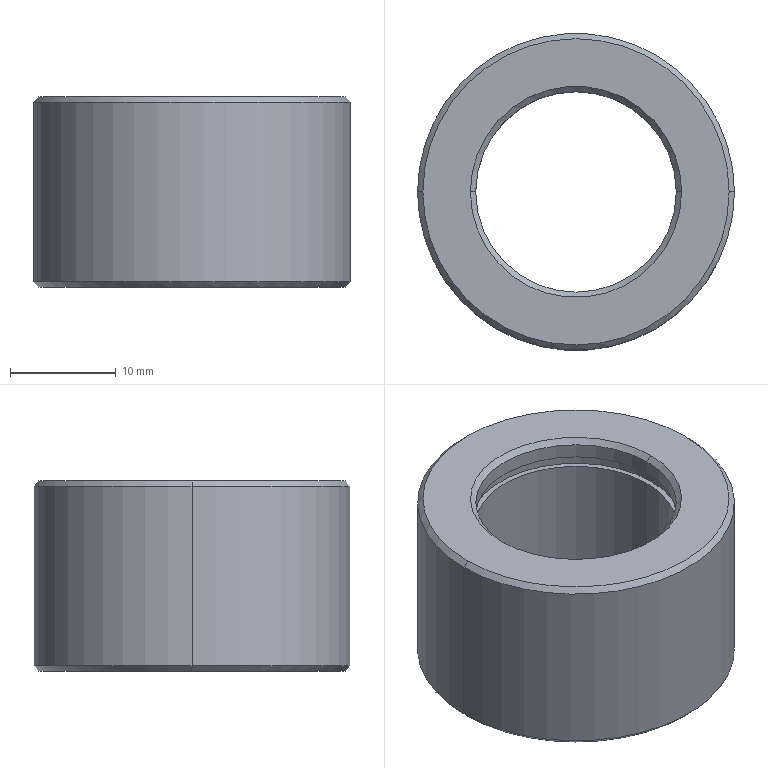Part | SolidWorks | features Chamfer 1, Extrusion 1, ICE 1, MirrorPattern 1 | 1 solid | 26 faces | box 30 x 30 x 18 mm | volume 7514 mm3 | cylinder 12 | cone 8 | plane 6 | commonest cylinder face diameters 19 x6 20 x4 30 x2
STEP:
#1=CARTESIAN_POINT('',(-9.5,0.,8.5));
#2=VERTEX_POINT('',#1);
#3=CARTESIAN_POINT('',(9.5,0.,8.5));
#4=VERTEX_POINT('',#3);
#5=CARTESIAN_POINT('',(0.,0.,8.5));
#6=DIRECTION('',(0.,0.,1.));
#7=DIRECTION('',(1.,0.,0.));
#8=AXIS2_PLACEMENT_3D('',#5,#6,#7);
#9=CIRCLE('',#8,9.5);
#10=EDGE_CURVE('',#2,#4,#9,.T.);
#11=ORIENTED_EDGE('',*,*,#10,.F.);
#12=CARTESIAN_POINT('',(-10.,0.,9.));
#13=VERTEX_POINT('',#12);
#14=CARTESIAN_POINT('',(-9.5,0.,8.5));
#15=DIRECTION('',(-0.7071,0.,0.7071));
#16=VECTOR('',#15,1000.);
#17=LINE('',#14,#16);
#18=EDGE_CURVE('',#2,#13,#17,.T.);
#19=ORIENTED_EDGE('',*,*,#18,.T.);
#20=CARTESIAN_POINT('',(10.,0.,9.));
#21=VERTEX_POINT('',#20);
#22=CARTESIAN_POINT('',(0.,0.,9.));
#23=DIRECTION('',(0.,0.,-1.));
#24=DIRECTION('',(1.,0.,0.));
#25=AXIS2_PLACEMENT_3D('',#22,#23,#24);
#26=CIRCLE('',#25,10.);
#27=EDGE_CURVE('',#21,#13,#26,.T.);
#28=ORIENTED_EDGE('',*,*,#27,.F.);
#29=CARTESIAN_POINT('',(9.5,0.,8.5));
#30=DIRECTION('',(0.7071,0.,0.7071));
#31=VECTOR('',#30,1000.);
#32=LINE('',#29,#31);
#33=EDGE_CURVE('',#4,#21,#32,.T.);
#34=ORIENTED_EDGE('',*,*,#33,.F.);
#35=EDGE_LOOP('',(#11,#19,#28,#34));
#36=FACE_OUTER_BOUND('',#35,.T.);
#37=CARTESIAN_POINT('',(0.,0.,8.5));
#38=DIRECTION('',(0.,0.,1.));
#39=DIRECTION('',(1.,0.,0.));
#40=AXIS2_PLACEMENT_3D('',#37,#38,#39);
#41=CONICAL_SURFACE('',#40,9.5,0.7854);
#42=ADVANCED_FACE('',(#36),#41,.F.);
#43=CARTESIAN_POINT('',(9.5,0.,-8.5));
#44=VERTEX_POINT('',#43);
#45=CARTESIAN_POINT('',(-9.5,0.,-8.5));
#46=VERTEX_POINT('',#45);
#47=CARTESIAN_POINT('',(0.,0.,-8.5));
#48=DIRECTION('',(0.,0.,-1.));
#49=DIRECTION('',(1.,0.,0.));
#50=AXIS2_PLACEMENT_3D('',#47,#48,#49);
#51=CIRCLE('',#50,9.5);
#52=EDGE_CURVE('',#44,#46,#51,.T.);
#53=ORIENTED_EDGE('',*,*,#52,.F.);
#54=CARTESIAN_POINT('',(10.,0.,-9.));
#55=VERTEX_POINT('',#54);
#56=CARTESIAN_POINT('',(10.,0.,-9.));
#57=DIRECTION('',(0.7071,0.,-0.7071));
#58=VECTOR('',#57,1000.);
#59=LINE('',#56,#58);
#60=EDGE_CURVE('',#44,#55,#59,.T.);
#61=ORIENTED_EDGE('',*,*,#60,.T.);
#62=CARTESIAN_POINT('',(-10.,0.,-9.));
#63=VERTEX_POINT('',#62);
#64=CARTESIAN_POINT('',(0.,0.,-9.));
#65=DIRECTION('',(0.,0.,1.));
#66=DIRECTION('',(1.,0.,0.));
#67=AXIS2_PLACEMENT_3D('',#64,#65,#66);
#68=CIRCLE('',#67,10.);
#69=EDGE_CURVE('',#63,#55,#68,.T.);
#70=ORIENTED_EDGE('',*,*,#69,.F.);
#71=CARTESIAN_POINT('',(-10.,0.,-9.));
#72=DIRECTION('',(-0.7071,0.,-0.7071));
#73=VECTOR('',#72,1000.);
#74=LINE('',#71,#73);
#75=EDGE_CURVE('',#46,#63,#74,.T.);
#76=ORIENTED_EDGE('',*,*,#75,.F.);
#77=EDGE_LOOP('',(#53,#61,#70,#76));
#78=FACE_OUTER_BOUND('',#77,.T.);
#79=CARTESIAN_POINT('',(0.,0.,-9.));
#80=DIRECTION('',(0.,0.,-1.));
#81=DIRECTION('',(-1.,0.,0.));
#82=AXIS2_PLACEMENT_3D('',#79,#80,#81);
#83=CONICAL_SURFACE('',#82,10.,0.7854);
#84=ADVANCED_FACE('',(#78),#83,.F.);
#85=CARTESIAN_POINT('',(14.5,0.,9.));
#86=VERTEX_POINT('',#85);
#87=CARTESIAN_POINT('',(-14.5,0.,9.));
#88=VERTEX_POINT('',#87);
#89=CARTESIAN_POINT('',(0.,0.,9.));
#90=DIRECTION('',(0.,0.,1.));
#91=DIRECTION('',(1.,0.,0.));
#92=AXIS2_PLACEMENT_3D('',#89,#90,#91);
#93=CIRCLE('',#92,14.5);
#94=EDGE_CURVE('',#86,#88,#93,.T.);
#95=ORIENTED_EDGE('',*,*,#94,.F.);
#96=CARTESIAN_POINT('',(15.,0.,8.5));
#97=VERTEX_POINT('',#96);
#98=CARTESIAN_POINT('',(14.5,0.,9.));
#99=DIRECTION('',(0.7071,0.,-0.7071));
#100=VECTOR('',#99,1000.);
#101=LINE('',#98,#100);
#102=EDGE_CURVE('',#86,#97,#101,.T.);
#103=ORIENTED_EDGE('',*,*,#102,.T.);
#104=CARTESIAN_POINT('',(-15.,0.,8.5));
#105=VERTEX_POINT('',#104);
#106=CARTESIAN_POINT('',(0.,0.,8.5));
#107=DIRECTION('',(0.,0.,-1.));
#108=DIRECTION('',(1.,0.,0.));
#109=AXIS2_PLACEMENT_3D('',#106,#107,#108);
#110=CIRCLE('',#109,15.);
#111=EDGE_CURVE('',#105,#97,#110,.T.);
#112=ORIENTED_EDGE('',*,*,#111,.F.);
#113=CARTESIAN_POINT('',(-14.5,0.,9.));
#114=DIRECTION('',(-0.7071,0.,-0.7071));
#115=VECTOR('',#114,1000.);
#116=LINE('',#113,#115);
#117=EDGE_CURVE('',#88,#105,#116,.T.);
#118=ORIENTED_EDGE('',*,*,#117,.F.);
#119=EDGE_LOOP('',(#95,#103,#112,#118));
#120=FACE_OUTER_BOUND('',#119,.T.);
#121=CARTESIAN_POINT('',(0.,0.,9.));
#122=DIRECTION('',(0.,0.,-1.));
#123=DIRECTION('',(-1.,0.,0.));
#124=AXIS2_PLACEMENT_3D('',#121,#122,#123);
#125=CONICAL_SURFACE('',#124,14.5,0.7854);
#126=ADVANCED_FACE('',(#120),#125,.T.);
#127=CARTESIAN_POINT('',(-14.5,0.,-9.));
#128=VERTEX_POINT('',#127);
#129=CARTESIAN_POINT('',(14.5,0.,-9.));
#130=VERTEX_POINT('',#129);
#131=CARTESIAN_POINT('',(0.,0.,-9.));
#132=DIRECTION('',(0.,0.,-1.));
#133=DIRECTION('',(1.,0.,0.));
#134=AXIS2_PLACEMENT_3D('',#131,#132,#133);
#135=CIRCLE('',#134,14.5);
#136=EDGE_CURVE('',#128,#130,#135,.T.);
#137=ORIENTED_EDGE('',*,*,#136,.F.);
#138=CARTESIAN_POINT('',(-15.,0.,-8.5));
#139=VERTEX_POINT('',#138);
#140=CARTESIAN_POINT('',(-15.,0.,-8.5));
#141=DIRECTION('',(-0.7071,0.,0.7071));
#142=VECTOR('',#141,1000.);
#143=LINE('',#140,#142);
#144=EDGE_CURVE('',#128,#139,#143,.T.);
#145=ORIENTED_EDGE('',*,*,#144,.T.);
#146=CARTESIAN_POINT('',(15.,0.,-8.5));
#147=VERTEX_POINT('',#146);
#148=CARTESIAN_POINT('',(0.,0.,-8.5));
#149=DIRECTION('',(0.,0.,1.));
#150=DIRECTION('',(1.,0.,0.));
#151=AXIS2_PLACEMENT_3D('',#148,#149,#150);
#152=CIRCLE('',#151,15.);
#153=EDGE_CURVE('',#147,#139,#152,.T.);
#154=ORIENTED_EDGE('',*,*,#153,.F.);
#155=CARTESIAN_POINT('',(15.,0.,-8.5));
#156=DIRECTION('',(0.7071,0.,0.7071));
#157=VECTOR('',#156,1000.);
#158=LINE('',#155,#157);
#159=EDGE_CURVE('',#130,#147,#158,.T.);
#160=ORIENTED_EDGE('',*,*,#159,.F.);
#161=EDGE_LOOP('',(#137,#145,#154,#160));
#162=FACE_OUTER_BOUND('',#161,.T.);
#163=CARTESIAN_POINT('',(0.,0.,-8.5));
#164=DIRECTION('',(0.,0.,1.));
#165=DIRECTION('',(1.,0.,0.));
#166=AXIS2_PLACEMENT_3D('',#163,#164,#165);
#167=CONICAL_SURFACE('',#166,15.,0.7854);
#168=ADVANCED_FACE('',(#162),#167,.T.);
#169=CARTESIAN_POINT('',(-10.,0.,-7.1));
#170=VERTEX_POINT('',#169);
#171=CARTESIAN_POINT('',(10.,0.,-7.1));
#172=VERTEX_POINT('',#171);
#173=CARTESIAN_POINT('',(0.,0.,-7.1));
#174=DIRECTION('',(0.,0.,1.));
#175=DIRECTION('',(1.,0.,0.));
#176=AXIS2_PLACEMENT_3D('',#173,#174,#175);
#177=CIRCLE('',#176,10.);
#178=EDGE_CURVE('',#170,#172,#177,.T.);
#179=ORIENTED_EDGE('',*,*,#178,.F.);
#180=CARTESIAN_POINT('',(-10.,0.,-6.));
#181=VERTEX_POINT('',#180);
#182=CARTESIAN_POINT('',(-10.,0.,-7.1));
#183=DIRECTION('',(0.,0.,1.));
#184=VECTOR('',#183,1000.);
#185=LINE('',#182,#184);
#186=EDGE_CURVE('',#170,#181,#185,.T.);
#187=ORIENTED_EDGE('',*,*,#186,.T.);
#188=CARTESIAN_POINT('',(10.,0.,-6.));
#189=VERTEX_POINT('',#188);
#190=CARTESIAN_POINT('',(0.,0.,-6.));
#191=DIRECTION('',(0.,0.,1.));
#192=DIRECTION('',(1.,0.,0.));
#193=AXIS2_PLACEMENT_3D('',#190,#191,#192);
#194=CIRCLE('',#193,10.);
#195=EDGE_CURVE('',#181,#189,#194,.T.);
#196=ORIENTED_EDGE('',*,*,#195,.T.);
#197=CARTESIAN_POINT('',(10.,0.,-7.1));
#198=DIRECTION('',(0.,0.,1.));
#199=VECTOR('',#198,1000.);
#200=LINE('',#197,#199);
#201=EDGE_CURVE('',#172,#189,#200,.T.);
#202=ORIENTED_EDGE('',*,*,#201,.F.);
#203=EDGE_LOOP('',(#179,#187,#196,#202));
#204=FACE_OUTER_BOUND('',#203,.T.);
#205=CARTESIAN_POINT('',(0.,0.,-7.1));
#206=DIRECTION('',(0.,0.,1.));
#207=DIRECTION('',(1.,0.,0.));
#208=AXIS2_PLACEMENT_3D('',#205,#206,#207);
#209=CYLINDRICAL_SURFACE('',#208,10.);
#210=ADVANCED_FACE('',(#204),#209,.F.);
#211=CARTESIAN_POINT('',(-10.,0.,7.1));
#212=VERTEX_POINT('',#211);
#213=CARTESIAN_POINT('',(10.,0.,7.1));
#214=VERTEX_POINT('',#213);
#215=CARTESIAN_POINT('',(0.,0.,7.1));
#216=DIRECTION('',(0.,0.,1.));
#217=DIRECTION('',(1.,0.,0.));
#218=AXIS2_PLACEMENT_3D('',#215,#216,#217);
#219=CIRCLE('',#218,10.);
#220=EDGE_CURVE('',#212,#214,#219,.T.);
#221=ORIENTED_EDGE('',*,*,#220,.T.);
#222=CARTESIAN_POINT('',(10.,0.,6.));
#223=VERTEX_POINT('',#222);
#224=CARTESIAN_POINT('',(10.,0.,7.1));
#225=DIRECTION('',(0.,0.,-1.));
#226=VECTOR('',#225,1000.);
#227=LINE('',#224,#226);
#228=EDGE_CURVE('',#214,#223,#227,.T.);
#229=ORIENTED_EDGE('',*,*,#228,.T.);
#230=CARTESIAN_POINT('',(-10.,0.,6.));
#231=VERTEX_POINT('',#230);
#232=CARTESIAN_POINT('',(0.,0.,6.));
#233=DIRECTION('',(0.,0.,1.));
#234=DIRECTION('',(1.,0.,0.));
#235=AXIS2_PLACEMENT_3D('',#232,#233,#234);
#236=CIRCLE('',#235,10.);
#237=EDGE_CURVE('',#231,#223,#236,.T.);
#238=ORIENTED_EDGE('',*,*,#237,.F.);
#239=CARTESIAN_POINT('',(-10.,0.,7.1));
#240=DIRECTION('',(0.,0.,-1.));
#241=VECTOR('',#240,1000.);
#242=LINE('',#239,#241);
#243=EDGE_CURVE('',#212,#231,#242,.T.);
#244=ORIENTED_EDGE('',*,*,#243,.F.);
#245=EDGE_LOOP('',(#221,#229,#238,#244));
#246=FACE_OUTER_BOUND('',#245,.T.);
#247=CARTESIAN_POINT('',(0.,0.,7.1));
#248=DIRECTION('',(0.,0.,-1.));
#249=DIRECTION('',(-1.,0.,0.));
#250=AXIS2_PLACEMENT_3D('',#247,#248,#249);
#251=CYLINDRICAL_SURFACE('',#250,10.);
#252=ADVANCED_FACE('',(#246),#251,.F.);
#253=ORIENTED_EDGE('',*,*,#10,.T.);
#254=CARTESIAN_POINT('',(9.5,0.,7.1));
#255=VERTEX_POINT('',#254);
#256=CARTESIAN_POINT('',(9.5,0.,9.));
#257=DIRECTION('',(0.,0.,-1.));
#258=VECTOR('',#257,1000.);
#259=LINE('',#256,#258);
#260=EDGE_CURVE('',#4,#255,#259,.T.);
#261=ORIENTED_EDGE('',*,*,#260,.T.);
#262=CARTESIAN_POINT('',(-9.5,0.,7.1));
#263=VERTEX_POINT('',#262);
#264=CARTESIAN_POINT('',(0.,0.,7.1));
#265=DIRECTION('',(0.,0.,1.));
#266=DIRECTION('',(1.,0.,0.));
#267=AXIS2_PLACEMENT_3D('',#264,#265,#266);
#268=CIRCLE('',#267,9.5);
#269=EDGE_CURVE('',#263,#255,#268,.T.);
#270=ORIENTED_EDGE('',*,*,#269,.F.);
#271=CARTESIAN_POINT('',(-9.5,0.,9.));
#272=DIRECTION('',(0.,0.,-1.));
#273=VECTOR('',#272,1000.);
#274=LINE('',#271,#273);
#275=EDGE_CURVE('',#2,#263,#274,.T.);
#276=ORIENTED_EDGE('',*,*,#275,.F.);
#277=EDGE_LOOP('',(#253,#261,#270,#276));
#278=FACE_OUTER_BOUND('',#277,.T.);
#279=CARTESIAN_POINT('',(0.,0.,9.));
#280=DIRECTION('',(0.,0.,-1.));
#281=DIRECTION('',(-1.,0.,0.));
#282=AXIS2_PLACEMENT_3D('',#279,#280,#281);
#283=CYLINDRICAL_SURFACE('',#282,9.5);
#284=ADVANCED_FACE('',(#278),#283,.F.);
#285=ORIENTED_EDGE('',*,*,#111,.T.);
#286=CARTESIAN_POINT('',(15.,0.,9.));
#287=DIRECTION('',(0.,0.,-1.));
#288=VECTOR('',#287,1000.);
#289=LINE('',#286,#288);
#290=EDGE_CURVE('',#97,#147,#289,.T.);
#291=ORIENTED_EDGE('',*,*,#290,.T.);
#292=ORIENTED_EDGE('',*,*,#153,.T.);
#293=CARTESIAN_POINT('',(-15.,0.,9.));
#294=DIRECTION('',(0.,0.,-1.));
#295=VECTOR('',#294,1000.);
#296=LINE('',#293,#295);
#297=EDGE_CURVE('',#105,#139,#296,.T.);
#298=ORIENTED_EDGE('',*,*,#297,.F.);
#299=EDGE_LOOP('',(#285,#291,#292,#298));
#300=FACE_OUTER_BOUND('',#299,.T.);
#301=CARTESIAN_POINT('',(0.,0.,9.));
#302=DIRECTION('',(0.,0.,-1.));
#303=DIRECTION('',(-1.,0.,0.));
#304=AXIS2_PLACEMENT_3D('',#301,#302,#303);
#305=CYLINDRICAL_SURFACE('',#304,15.);
#306=ADVANCED_FACE('',(#300),#305,.T.);
#307=CARTESIAN_POINT('',(-9.5,0.,-7.1));
#308=VERTEX_POINT('',#307);
#309=CARTESIAN_POINT('',(9.5,0.,-7.1));
#310=VERTEX_POINT('',#309);
#311=CARTESIAN_POINT('',(0.,0.,-7.1));
#312=DIRECTION('',(0.,0.,1.));
#313=DIRECTION('',(1.,0.,0.));
#314=AXIS2_PLACEMENT_3D('',#311,#312,#313);
#315=CIRCLE('',#314,9.5);
#316=EDGE_CURVE('',#308,#310,#315,.T.);
#317=ORIENTED_EDGE('',*,*,#316,.T.);
#318=CARTESIAN_POINT('',(9.5,0.,9.));
#319=DIRECTION('',(0.,0.,-1.));
#320=VECTOR('',#319,1000.);
#321=LINE('',#318,#320);
#322=EDGE_CURVE('',#310,#44,#321,.T.);
#323=ORIENTED_EDGE('',*,*,#322,.T.);
#324=ORIENTED_EDGE('',*,*,#52,.T.);
#325=CARTESIAN_POINT('',(-9.5,0.,9.));
#326=DIRECTION('',(0.,0.,-1.));
#327=VECTOR('',#326,1000.);
#328=LINE('',#325,#327);
#329=EDGE_CURVE('',#308,#46,#328,.T.);
#330=ORIENTED_EDGE('',*,*,#329,.F.);
#331=EDGE_LOOP('',(#317,#323,#324,#330));
#332=FACE_OUTER_BOUND('',#331,.T.);
#333=CARTESIAN_POINT('',(0.,0.,9.));
#334=DIRECTION('',(0.,0.,-1.));
#335=DIRECTION('',(-1.,0.,0.));
#336=AXIS2_PLACEMENT_3D('',#333,#334,#335);
#337=CYLINDRICAL_SURFACE('',#336,9.5);
#338=ADVANCED_FACE('',(#332),#337,.F.);
#339=CARTESIAN_POINT('',(-9.5,0.,6.));
#340=VERTEX_POINT('',#339);
#341=CARTESIAN_POINT('',(9.5,0.,6.));
#342=VERTEX_POINT('',#341);
#343=CARTESIAN_POINT('',(0.,0.,6.));
#344=DIRECTION('',(0.,0.,1.));
#345=DIRECTION('',(1.,0.,0.));
#346=AXIS2_PLACEMENT_3D('',#343,#344,#345);
#347=CIRCLE('',#346,9.5);
#348=EDGE_CURVE('',#340,#342,#347,.T.);
#349=ORIENTED_EDGE('',*,*,#348,.T.);
#350=CARTESIAN_POINT('',(9.5,0.,-6.));
#351=VERTEX_POINT('',#350);
#352=CARTESIAN_POINT('',(9.5,0.,9.));
#353=DIRECTION('',(0.,0.,-1.));
#354=VECTOR('',#353,1000.);
#355=LINE('',#352,#354);
#356=EDGE_CURVE('',#342,#351,#355,.T.);
#357=ORIENTED_EDGE('',*,*,#356,.T.);
#358=CARTESIAN_POINT('',(-9.5,0.,-6.));
#359=VERTEX_POINT('',#358);
#360=CARTESIAN_POINT('',(0.,0.,-6.));
#361=DIRECTION('',(0.,0.,1.));
#362=DIRECTION('',(1.,0.,0.));
#363=AXIS2_PLACEMENT_3D('',#360,#361,#362);
#364=CIRCLE('',#363,9.5);
#365=EDGE_CURVE('',#359,#351,#364,.T.);
#366=ORIENTED_EDGE('',*,*,#365,.F.);
#367=CARTESIAN_POINT('',(-9.5,0.,9.));
#368=DIRECTION('',(0.,0.,-1.));
#369=VECTOR('',#368,1000.);
#370=LINE('',#367,#369);
#371=EDGE_CURVE('',#340,#359,#370,.T.);
#372=ORIENTED_EDGE('',*,*,#371,.F.);
#373=EDGE_LOOP('',(#349,#357,#366,#372));
#374=FACE_OUTER_BOUND('',#373,.T.);
#375=CARTESIAN_POINT('',(0.,0.,9.));
#376=DIRECTION('',(0.,0.,-1.));
#377=DIRECTION('',(-1.,0.,0.));
#378=AXIS2_PLACEMENT_3D('',#375,#376,#377);
#379=CYLINDRICAL_SURFACE('',#378,9.5);
#380=ADVANCED_FACE('',(#374),#379,.F.);
#381=ORIENTED_EDGE('',*,*,#356,.F.);
#382=CARTESIAN_POINT('',(0.,0.,6.));
#383=DIRECTION('',(0.,0.,1.));
#384=DIRECTION('',(1.,0.,0.));
#385=AXIS2_PLACEMENT_3D('',#382,#383,#384);
#386=CIRCLE('',#385,9.5);
#387=EDGE_CURVE('',#342,#340,#386,.T.);
#388=ORIENTED_EDGE('',*,*,#387,.T.);
#389=ORIENTED_EDGE('',*,*,#371,.T.);
#390=CARTESIAN_POINT('',(0.,0.,-6.));
#391=DIRECTION('',(0.,0.,1.));
#392=DIRECTION('',(1.,0.,0.));
#393=AXIS2_PLACEMENT_3D('',#390,#391,#392);
#394=CIRCLE('',#393,9.5);
#395=EDGE_CURVE('',#351,#359,#394,.T.);
#396=ORIENTED_EDGE('',*,*,#395,.F.);
#397=EDGE_LOOP('',(#381,#388,#389,#396));
#398=FACE_OUTER_BOUND('',#397,.T.);
#399=CARTESIAN_POINT('',(0.,0.,9.));
#400=DIRECTION('',(0.,0.,-1.));
#401=DIRECTION('',(-1.,0.,0.));
#402=AXIS2_PLACEMENT_3D('',#399,#400,#401);
#403=CYLINDRICAL_SURFACE('',#402,9.5);
#404=ADVANCED_FACE('',(#398),#403,.F.);
#405=ORIENTED_EDGE('',*,*,#322,.F.);
#406=CARTESIAN_POINT('',(0.,0.,-7.1));
#407=DIRECTION('',(0.,0.,1.));
#408=DIRECTION('',(1.,0.,0.));
#409=AXIS2_PLACEMENT_3D('',#406,#407,#408);
#410=CIRCLE('',#409,9.5);
#411=EDGE_CURVE('',#310,#308,#410,.T.);
#412=ORIENTED_EDGE('',*,*,#411,.T.);
#413=ORIENTED_EDGE('',*,*,#329,.T.);
#414=CARTESIAN_POINT('',(0.,0.,-8.5));
#415=DIRECTION('',(0.,0.,-1.));
#416=DIRECTION('',(1.,0.,0.));
#417=AXIS2_PLACEMENT_3D('',#414,#415,#416);
#418=CIRCLE('',#417,9.5);
#419=EDGE_CURVE('',#46,#44,#418,.T.);
#420=ORIENTED_EDGE('',*,*,#419,.T.);
#421=EDGE_LOOP('',(#405,#412,#413,#420));
#422=FACE_OUTER_BOUND('',#421,.T.);
#423=CARTESIAN_POINT('',(0.,0.,9.));
#424=DIRECTION('',(0.,0.,-1.));
#425=DIRECTION('',(-1.,0.,0.));
#426=AXIS2_PLACEMENT_3D('',#423,#424,#425);
#427=CYLINDRICAL_SURFACE('',#426,9.5);
#428=ADVANCED_FACE('',(#422),#427,.F.);
#429=CARTESIAN_POINT('',(0.,0.,9.));
#430=DIRECTION('',(0.,0.,1.));
#431=DIRECTION('',(1.,0.,0.));
#432=AXIS2_PLACEMENT_3D('',#429,#430,#431);
#433=CIRCLE('',#432,14.5);
#434=EDGE_CURVE('',#88,#86,#433,.T.);
#435=ORIENTED_EDGE('',*,*,#434,.T.);
#436=ORIENTED_EDGE('',*,*,#94,.T.);
#437=EDGE_LOOP('',(#435,#436));
#438=FACE_OUTER_BOUND('',#437,.T.);
#439=ORIENTED_EDGE('',*,*,#27,.T.);
#440=CARTESIAN_POINT('',(0.,0.,9.));
#441=DIRECTION('',(0.,0.,-1.));
#442=DIRECTION('',(1.,0.,0.));
#443=AXIS2_PLACEMENT_3D('',#440,#441,#442);
#444=CIRCLE('',#443,10.);
#445=EDGE_CURVE('',#13,#21,#444,.T.);
#446=ORIENTED_EDGE('',*,*,#445,.T.);
#447=EDGE_LOOP('',(#439,#446));
#448=FACE_BOUND('',#447,.T.);
#449=CARTESIAN_POINT('',(0.,0.,9.));
#450=DIRECTION('',(0.,0.,1.));
#451=DIRECTION('',(1.,0.,0.));
#452=AXIS2_PLACEMENT_3D('',#449,#450,#451);
#453=PLANE('',#452);
#454=ADVANCED_FACE('',(#438,#448),#453,.T.);
#455=CARTESIAN_POINT('',(0.,0.,-9.));
#456=DIRECTION('',(0.,0.,-1.));
#457=DIRECTION('',(1.,0.,0.));
#458=AXIS2_PLACEMENT_3D('',#455,#456,#457);
#459=CIRCLE('',#458,14.5);
#460=EDGE_CURVE('',#130,#128,#459,.T.);
#461=ORIENTED_EDGE('',*,*,#460,.T.);
#462=ORIENTED_EDGE('',*,*,#136,.T.);
#463=EDGE_LOOP('',(#461,#462));
#464=FACE_OUTER_BOUND('',#463,.T.);
#465=ORIENTED_EDGE('',*,*,#69,.T.);
#466=CARTESIAN_POINT('',(0.,0.,-9.));
#467=DIRECTION('',(0.,0.,1.));
#468=DIRECTION('',(1.,0.,0.));
#469=AXIS2_PLACEMENT_3D('',#466,#467,#468);
#470=CIRCLE('',#469,10.);
#471=EDGE_CURVE('',#55,#63,#470,.T.);
#472=ORIENTED_EDGE('',*,*,#471,.T.);
#473=EDGE_LOOP('',(#465,#472));
#474=FACE_BOUND('',#473,.T.);
#475=CARTESIAN_POINT('',(0.,0.,-9.));
#476=DIRECTION('',(0.,0.,1.));
#477=DIRECTION('',(1.,0.,0.));
#478=AXIS2_PLACEMENT_3D('',#475,#476,#477);
#479=PLANE('',#478);
#480=ADVANCED_FACE('',(#464,#474),#479,.F.);
#481=ORIENTED_EDGE('',*,*,#290,.F.);
#482=CARTESIAN_POINT('',(0.,0.,8.5));
#483=DIRECTION('',(0.,0.,-1.));
#484=DIRECTION('',(1.,0.,0.));
#485=AXIS2_PLACEMENT_3D('',#482,#483,#484);
#486=CIRCLE('',#485,15.);
#487=EDGE_CURVE('',#97,#105,#486,.T.);
#488=ORIENTED_EDGE('',*,*,#487,.T.);
#489=ORIENTED_EDGE('',*,*,#297,.T.);
#490=CARTESIAN_POINT('',(0.,0.,-8.5));
#491=DIRECTION('',(0.,0.,1.));
#492=DIRECTION('',(1.,0.,0.));
#493=AXIS2_PLACEMENT_3D('',#490,#491,#492);
#494=CIRCLE('',#493,15.);
#495=EDGE_CURVE('',#139,#147,#494,.T.);
#496=ORIENTED_EDGE('',*,*,#495,.T.);
#497=EDGE_LOOP('',(#481,#488,#489,#496));
#498=FACE_OUTER_BOUND('',#497,.T.);
#499=CARTESIAN_POINT('',(0.,0.,9.));
#500=DIRECTION('',(0.,0.,-1.));
#501=DIRECTION('',(-1.,0.,0.));
#502=AXIS2_PLACEMENT_3D('',#499,#500,#501);
#503=CYLINDRICAL_SURFACE('',#502,15.);
#504=ADVANCED_FACE('',(#498),#503,.T.);
#505=ORIENTED_EDGE('',*,*,#260,.F.);
#506=CARTESIAN_POINT('',(0.,0.,8.5));
#507=DIRECTION('',(0.,0.,1.));
#508=DIRECTION('',(1.,0.,0.));
#509=AXIS2_PLACEMENT_3D('',#506,#507,#508);
#510=CIRCLE('',#509,9.5);
#511=EDGE_CURVE('',#4,#2,#510,.T.);
#512=ORIENTED_EDGE('',*,*,#511,.T.);
#513=ORIENTED_EDGE('',*,*,#275,.T.);
#514=CARTESIAN_POINT('',(0.,0.,7.1));
#515=DIRECTION('',(0.,0.,1.));
#516=DIRECTION('',(1.,0.,0.));
#517=AXIS2_PLACEMENT_3D('',#514,#515,#516);
#518=CIRCLE('',#517,9.5);
#519=EDGE_CURVE('',#255,#263,#518,.T.);
#520=ORIENTED_EDGE('',*,*,#519,.F.);
#521=EDGE_LOOP('',(#505,#512,#513,#520));
#522=FACE_OUTER_BOUND('',#521,.T.);
#523=CARTESIAN_POINT('',(0.,0.,9.));
#524=DIRECTION('',(0.,0.,-1.));
#525=DIRECTION('',(-1.,0.,0.));
#526=AXIS2_PLACEMENT_3D('',#523,#524,#525);
#527=CYLINDRICAL_SURFACE('',#526,9.5);
#528=ADVANCED_FACE('',(#522),#527,.F.);
#529=ORIENTED_EDGE('',*,*,#220,.F.);
#530=CARTESIAN_POINT('',(0.,0.,7.1));
#531=DIRECTION('',(0.,0.,1.));
#532=DIRECTION('',(1.,0.,0.));
#533=AXIS2_PLACEMENT_3D('',#530,#531,#532);
#534=CIRCLE('',#533,10.);
#535=EDGE_CURVE('',#214,#212,#534,.T.);
#536=ORIENTED_EDGE('',*,*,#535,.F.);
#537=EDGE_LOOP('',(#529,#536));
#538=FACE_OUTER_BOUND('',#537,.T.);
#539=ORIENTED_EDGE('',*,*,#269,.T.);
#540=ORIENTED_EDGE('',*,*,#519,.T.);
#541=EDGE_LOOP('',(#539,#540));
#542=FACE_BOUND('',#541,.T.);
#543=CARTESIAN_POINT('',(0.,0.,7.1));
#544=DIRECTION('',(0.,0.,1.));
#545=DIRECTION('',(1.,0.,0.));
#546=AXIS2_PLACEMENT_3D('',#543,#544,#545);
#547=PLANE('',#546);
#548=ADVANCED_FACE('',(#538,#542),#547,.F.);
#549=ORIENTED_EDGE('',*,*,#237,.T.);
#550=CARTESIAN_POINT('',(0.,0.,6.));
#551=DIRECTION('',(0.,0.,1.));
#552=DIRECTION('',(1.,0.,0.));
#553=AXIS2_PLACEMENT_3D('',#550,#551,#552);
#554=CIRCLE('',#553,10.);
#555=EDGE_CURVE('',#223,#231,#554,.T.);
#556=ORIENTED_EDGE('',*,*,#555,.T.);
#557=EDGE_LOOP('',(#549,#556));
#558=FACE_OUTER_BOUND('',#557,.T.);
#559=ORIENTED_EDGE('',*,*,#348,.F.);
#560=ORIENTED_EDGE('',*,*,#387,.F.);
#561=EDGE_LOOP('',(#559,#560));
#562=FACE_BOUND('',#561,.T.);
#563=CARTESIAN_POINT('',(0.,0.,6.));
#564=DIRECTION('',(0.,0.,1.));
#565=DIRECTION('',(1.,0.,0.));
#566=AXIS2_PLACEMENT_3D('',#563,#564,#565);
#567=PLANE('',#566);
#568=ADVANCED_FACE('',(#558,#562),#567,.T.);
#569=ORIENTED_EDGE('',*,*,#228,.F.);
#570=ORIENTED_EDGE('',*,*,#535,.T.);
#571=ORIENTED_EDGE('',*,*,#243,.T.);
#572=ORIENTED_EDGE('',*,*,#555,.F.);
#573=EDGE_LOOP('',(#569,#570,#571,#572));
#574=FACE_OUTER_BOUND('',#573,.T.);
#575=CARTESIAN_POINT('',(0.,0.,7.1));
#576=DIRECTION('',(0.,0.,-1.));
#577=DIRECTION('',(-1.,0.,0.));
#578=AXIS2_PLACEMENT_3D('',#575,#576,#577);
#579=CYLINDRICAL_SURFACE('',#578,10.);
#580=ADVANCED_FACE('',(#574),#579,.F.);
#581=ORIENTED_EDGE('',*,*,#186,.F.);
#582=CARTESIAN_POINT('',(0.,0.,-7.1));
#583=DIRECTION('',(0.,0.,1.));
#584=DIRECTION('',(1.,0.,0.));
#585=AXIS2_PLACEMENT_3D('',#582,#583,#584);
#586=CIRCLE('',#585,10.);
#587=EDGE_CURVE('',#172,#170,#586,.T.);
#588=ORIENTED_EDGE('',*,*,#587,.F.);
#589=ORIENTED_EDGE('',*,*,#201,.T.);
#590=CARTESIAN_POINT('',(0.,0.,-6.));
#591=DIRECTION('',(0.,0.,1.));
#592=DIRECTION('',(1.,0.,0.));
#593=AXIS2_PLACEMENT_3D('',#590,#591,#592);
#594=CIRCLE('',#593,10.);
#595=EDGE_CURVE('',#189,#181,#594,.T.);
#596=ORIENTED_EDGE('',*,*,#595,.T.);
#597=EDGE_LOOP('',(#581,#588,#589,#596));
#598=FACE_OUTER_BOUND('',#597,.T.);
#599=CARTESIAN_POINT('',(0.,0.,-7.1));
#600=DIRECTION('',(0.,0.,1.));
#601=DIRECTION('',(1.,0.,0.));
#602=AXIS2_PLACEMENT_3D('',#599,#600,#601);
#603=CYLINDRICAL_SURFACE('',#602,10.);
#604=ADVANCED_FACE('',(#598),#603,.F.);
#605=ORIENTED_EDGE('',*,*,#316,.F.);
#606=ORIENTED_EDGE('',*,*,#411,.F.);
#607=EDGE_LOOP('',(#605,#606));
#608=FACE_BOUND('',#607,.T.);
#609=ORIENTED_EDGE('',*,*,#587,.T.);
#610=ORIENTED_EDGE('',*,*,#178,.T.);
#611=EDGE_LOOP('',(#609,#610));
#612=FACE_OUTER_BOUND('',#611,.T.);
#613=CARTESIAN_POINT('',(0.,0.,-7.1));
#614=DIRECTION('',(0.,0.,-1.));
#615=DIRECTION('',(1.,0.,0.));
#616=AXIS2_PLACEMENT_3D('',#613,#614,#615);
#617=PLANE('',#616);
#618=ADVANCED_FACE('',(#608,#612),#617,.F.);
#619=ORIENTED_EDGE('',*,*,#365,.T.);
#620=ORIENTED_EDGE('',*,*,#395,.T.);
#621=EDGE_LOOP('',(#619,#620));
#622=FACE_BOUND('',#621,.T.);
#623=ORIENTED_EDGE('',*,*,#595,.F.);
#624=ORIENTED_EDGE('',*,*,#195,.F.);
#625=EDGE_LOOP('',(#623,#624));
#626=FACE_OUTER_BOUND('',#625,.T.);
#627=CARTESIAN_POINT('',(0.,0.,-6.));
#628=DIRECTION('',(0.,0.,-1.));
#629=DIRECTION('',(1.,0.,0.));
#630=AXIS2_PLACEMENT_3D('',#627,#628,#629);
#631=PLANE('',#630);
#632=ADVANCED_FACE('',(#622,#626),#631,.T.);
#633=ORIENTED_EDGE('',*,*,#144,.F.);
#634=ORIENTED_EDGE('',*,*,#460,.F.);
#635=ORIENTED_EDGE('',*,*,#159,.T.);
#636=ORIENTED_EDGE('',*,*,#495,.F.);
#637=EDGE_LOOP('',(#633,#634,#635,#636));
#638=FACE_OUTER_BOUND('',#637,.T.);
#639=CARTESIAN_POINT('',(0.,0.,-8.5));
#640=DIRECTION('',(0.,0.,1.));
#641=DIRECTION('',(1.,0.,0.));
#642=AXIS2_PLACEMENT_3D('',#639,#640,#641);
#643=CONICAL_SURFACE('',#642,15.,0.7854);
#644=ADVANCED_FACE('',(#638),#643,.T.);
#645=ORIENTED_EDGE('',*,*,#102,.F.);
#646=ORIENTED_EDGE('',*,*,#434,.F.);
#647=ORIENTED_EDGE('',*,*,#117,.T.);
#648=ORIENTED_EDGE('',*,*,#487,.F.);
#649=EDGE_LOOP('',(#645,#646,#647,#648));
#650=FACE_OUTER_BOUND('',#649,.T.);
#651=CARTESIAN_POINT('',(0.,0.,9.));
#652=DIRECTION('',(0.,0.,-1.));
#653=DIRECTION('',(-1.,0.,0.));
#654=AXIS2_PLACEMENT_3D('',#651,#652,#653);
#655=CONICAL_SURFACE('',#654,14.5,0.7854);
#656=ADVANCED_FACE('',(#650),#655,.T.);
#657=ORIENTED_EDGE('',*,*,#60,.F.);
#658=ORIENTED_EDGE('',*,*,#419,.F.);
#659=ORIENTED_EDGE('',*,*,#75,.T.);
#660=ORIENTED_EDGE('',*,*,#471,.F.);
#661=EDGE_LOOP('',(#657,#658,#659,#660));
#662=FACE_OUTER_BOUND('',#661,.T.);
#663=CARTESIAN_POINT('',(0.,0.,-9.));
#664=DIRECTION('',(0.,0.,-1.));
#665=DIRECTION('',(-1.,0.,0.));
#666=AXIS2_PLACEMENT_3D('',#663,#664,#665);
#667=CONICAL_SURFACE('',#666,10.,0.7854);
#668=ADVANCED_FACE('',(#662),#667,.F.);
#669=ORIENTED_EDGE('',*,*,#18,.F.);
#670=ORIENTED_EDGE('',*,*,#511,.F.);
#671=ORIENTED_EDGE('',*,*,#33,.T.);
#672=ORIENTED_EDGE('',*,*,#445,.F.);
#673=EDGE_LOOP('',(#669,#670,#671,#672));
#674=FACE_OUTER_BOUND('',#673,.T.);
#675=CARTESIAN_POINT('',(0.,0.,8.5));
#676=DIRECTION('',(0.,0.,1.));
#677=DIRECTION('',(1.,0.,0.));
#678=AXIS2_PLACEMENT_3D('',#675,#676,#677);
#679=CONICAL_SURFACE('',#678,9.5,0.7854);
#680=ADVANCED_FACE('',(#674),#679,.F.);
#681=CLOSED_SHELL('',(#42,#84,#126,#168,#210,#252,#284,#306,#338,#380,#404,#428,#454,#480,#504,#528,#548,#568,#580,#604,#618,#632,#644,#656,#668,#680));
#682=MANIFOLD_SOLID_BREP('',#681);
#683=CARTESIAN_POINT('',(0.,0.,0.));
#684=DIRECTION('',(0.,0.,1.));
#685=DIRECTION('',(1.,0.,0.));
#686=AXIS2_PLACEMENT_3D('',#683,#684,#685);
#687=(LENGTH_UNIT()NAMED_UNIT(*)SI_UNIT(.MILLI.,.METRE.));
#688=UNCERTAINTY_MEASURE_WITH_UNIT(LENGTH_MEASURE(0.00001),#687,'','');
#689=(NAMED_UNIT(*)PLANE_ANGLE_UNIT()SI_UNIT($,.RADIAN.));
#690=(NAMED_UNIT(*)SI_UNIT($,.STERADIAN.)SOLID_ANGLE_UNIT());
#691=(GEOMETRIC_REPRESENTATION_CONTEXT(3)GLOBAL_UNCERTAINTY_ASSIGNED_CONTEXT((#688))GLOBAL_UNIT_ASSIGNED_CONTEXT((#687,#689,#690))REPRESENTATION_CONTEXT('',''));
#692=ADVANCED_BREP_SHAPE_REPRESENTATION('',(#682,#686),#691);